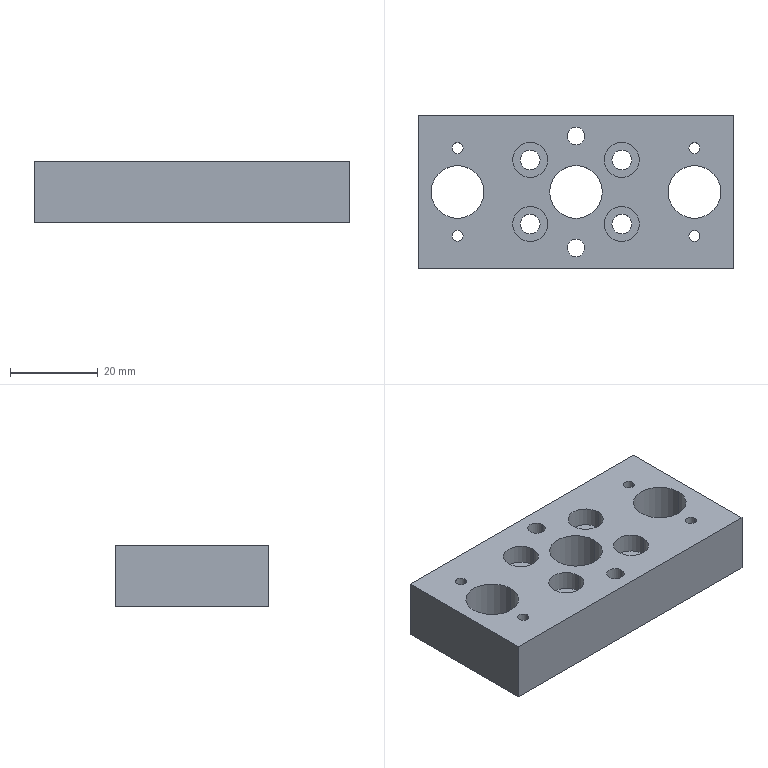Part | STEP file | 11-FG-SB01111 | 1 solid | 44 faces | box 72 x 35 x 14 mm | volume 28408 mm3 | cylinder 34 | plane 10 | commonest cylinder face diameters 2.5 x8 4.5 x8 8 x8 12 x6 4 x4
STEP:
#1=CARTESIAN_POINT('',(-6.,0.,0.));
#2=VERTEX_POINT('',#1);
#3=CARTESIAN_POINT('',(6.,0.,0.));
#4=VERTEX_POINT('',#3);
#5=CARTESIAN_POINT('',(0.,0.,0.));
#6=DIRECTION('',(0.,0.,1.));
#7=DIRECTION('',(1.,0.,0.));
#8=AXIS2_PLACEMENT_3D('',#5,#6,#7);
#9=CIRCLE('',#8,6.);
#10=EDGE_CURVE('',#2,#4,#9,.T.);
#11=ORIENTED_EDGE('',*,*,#10,.F.);
#12=CARTESIAN_POINT('',(-6.,0.,14.));
#13=VERTEX_POINT('',#12);
#14=CARTESIAN_POINT('',(-6.,0.,0.));
#15=DIRECTION('',(0.,0.,1.));
#16=VECTOR('',#15,1000.);
#17=LINE('',#14,#16);
#18=EDGE_CURVE('',#2,#13,#17,.T.);
#19=ORIENTED_EDGE('',*,*,#18,.T.);
#20=CARTESIAN_POINT('',(6.,0.,14.));
#21=VERTEX_POINT('',#20);
#22=CARTESIAN_POINT('',(0.,0.,14.));
#23=DIRECTION('',(0.,0.,1.));
#24=DIRECTION('',(1.,0.,0.));
#25=AXIS2_PLACEMENT_3D('',#22,#23,#24);
#26=CIRCLE('',#25,6.);
#27=EDGE_CURVE('',#13,#21,#26,.T.);
#28=ORIENTED_EDGE('',*,*,#27,.T.);
#29=CARTESIAN_POINT('',(6.,0.,0.));
#30=DIRECTION('',(0.,0.,1.));
#31=VECTOR('',#30,1000.);
#32=LINE('',#29,#31);
#33=EDGE_CURVE('',#4,#21,#32,.T.);
#34=ORIENTED_EDGE('',*,*,#33,.F.);
#35=EDGE_LOOP('',(#11,#19,#28,#34));
#36=FACE_OUTER_BOUND('',#35,.T.);
#37=CARTESIAN_POINT('',(0.,0.,0.));
#38=DIRECTION('',(0.,0.,1.));
#39=DIRECTION('',(1.,0.,0.));
#40=AXIS2_PLACEMENT_3D('',#37,#38,#39);
#41=CYLINDRICAL_SURFACE('',#40,6.);
#42=ADVANCED_FACE('',(#36),#41,.F.);
#43=CARTESIAN_POINT('',(28.25,10.,14.));
#44=VERTEX_POINT('',#43);
#45=CARTESIAN_POINT('',(25.75,10.,14.));
#46=VERTEX_POINT('',#45);
#47=CARTESIAN_POINT('',(27.,10.,14.));
#48=DIRECTION('',(0.,0.,-1.));
#49=DIRECTION('',(-1.,0.,0.));
#50=AXIS2_PLACEMENT_3D('',#47,#48,#49);
#51=CIRCLE('',#50,1.25);
#52=EDGE_CURVE('',#44,#46,#51,.T.);
#53=ORIENTED_EDGE('',*,*,#52,.F.);
#54=CARTESIAN_POINT('',(28.25,10.,0.));
#55=VERTEX_POINT('',#54);
#56=CARTESIAN_POINT('',(28.25,10.,0.));
#57=DIRECTION('',(0.,0.,-1.));
#58=VECTOR('',#57,1000.);
#59=LINE('',#56,#58);
#60=EDGE_CURVE('',#44,#55,#59,.T.);
#61=ORIENTED_EDGE('',*,*,#60,.T.);
#62=CARTESIAN_POINT('',(25.75,10.,0.));
#63=VERTEX_POINT('',#62);
#64=CARTESIAN_POINT('',(27.,10.,0.));
#65=DIRECTION('',(0.,0.,-1.));
#66=DIRECTION('',(-1.,0.,0.));
#67=AXIS2_PLACEMENT_3D('',#64,#65,#66);
#68=CIRCLE('',#67,1.25);
#69=EDGE_CURVE('',#55,#63,#68,.T.);
#70=ORIENTED_EDGE('',*,*,#69,.T.);
#71=CARTESIAN_POINT('',(25.75,10.,0.));
#72=DIRECTION('',(0.,0.,-1.));
#73=VECTOR('',#72,1000.);
#74=LINE('',#71,#73);
#75=EDGE_CURVE('',#46,#63,#74,.T.);
#76=ORIENTED_EDGE('',*,*,#75,.F.);
#77=EDGE_LOOP('',(#53,#61,#70,#76));
#78=FACE_OUTER_BOUND('',#77,.T.);
#79=CARTESIAN_POINT('',(27.,10.,0.));
#80=DIRECTION('',(0.,0.,-1.));
#81=DIRECTION('',(-1.,0.,0.));
#82=AXIS2_PLACEMENT_3D('',#79,#80,#81);
#83=CYLINDRICAL_SURFACE('',#82,1.25);
#84=ADVANCED_FACE('',(#78),#83,.F.);
#85=CARTESIAN_POINT('',(28.25,-10.018,14.));
#86=VERTEX_POINT('',#85);
#87=CARTESIAN_POINT('',(25.75,-10.018,14.));
#88=VERTEX_POINT('',#87);
#89=CARTESIAN_POINT('',(27.,-10.018,14.));
#90=DIRECTION('',(0.,0.,-1.));
#91=DIRECTION('',(-1.,0.,0.));
#92=AXIS2_PLACEMENT_3D('',#89,#90,#91);
#93=CIRCLE('',#92,1.25);
#94=EDGE_CURVE('',#86,#88,#93,.T.);
#95=ORIENTED_EDGE('',*,*,#94,.F.);
#96=CARTESIAN_POINT('',(28.25,-10.018,0.));
#97=VERTEX_POINT('',#96);
#98=CARTESIAN_POINT('',(28.25,-10.018,0.));
#99=DIRECTION('',(0.,0.,-1.));
#100=VECTOR('',#99,1000.);
#101=LINE('',#98,#100);
#102=EDGE_CURVE('',#86,#97,#101,.T.);
#103=ORIENTED_EDGE('',*,*,#102,.T.);
#104=CARTESIAN_POINT('',(25.75,-10.018,0.));
#105=VERTEX_POINT('',#104);
#106=CARTESIAN_POINT('',(27.,-10.018,0.));
#107=DIRECTION('',(0.,0.,-1.));
#108=DIRECTION('',(-1.,0.,0.));
#109=AXIS2_PLACEMENT_3D('',#106,#107,#108);
#110=CIRCLE('',#109,1.25);
#111=EDGE_CURVE('',#97,#105,#110,.T.);
#112=ORIENTED_EDGE('',*,*,#111,.T.);
#113=CARTESIAN_POINT('',(25.75,-10.018,0.));
#114=DIRECTION('',(0.,0.,-1.));
#115=VECTOR('',#114,1000.);
#116=LINE('',#113,#115);
#117=EDGE_CURVE('',#88,#105,#116,.T.);
#118=ORIENTED_EDGE('',*,*,#117,.F.);
#119=EDGE_LOOP('',(#95,#103,#112,#118));
#120=FACE_OUTER_BOUND('',#119,.T.);
#121=CARTESIAN_POINT('',(27.,-10.018,0.));
#122=DIRECTION('',(0.,0.,-1.));
#123=DIRECTION('',(-1.,0.,0.));
#124=AXIS2_PLACEMENT_3D('',#121,#122,#123);
#125=CYLINDRICAL_SURFACE('',#124,1.25);
#126=ADVANCED_FACE('',(#120),#125,.F.);
#127=CARTESIAN_POINT('',(-25.75,10.,14.));
#128=VERTEX_POINT('',#127);
#129=CARTESIAN_POINT('',(-28.25,10.,14.));
#130=VERTEX_POINT('',#129);
#131=CARTESIAN_POINT('',(-27.,10.,14.));
#132=DIRECTION('',(0.,0.,-1.));
#133=DIRECTION('',(-1.,0.,0.));
#134=AXIS2_PLACEMENT_3D('',#131,#132,#133);
#135=CIRCLE('',#134,1.25);
#136=EDGE_CURVE('',#128,#130,#135,.T.);
#137=ORIENTED_EDGE('',*,*,#136,.F.);
#138=CARTESIAN_POINT('',(-25.75,10.,0.));
#139=VERTEX_POINT('',#138);
#140=CARTESIAN_POINT('',(-25.75,10.,0.));
#141=DIRECTION('',(0.,0.,-1.));
#142=VECTOR('',#141,1000.);
#143=LINE('',#140,#142);
#144=EDGE_CURVE('',#128,#139,#143,.T.);
#145=ORIENTED_EDGE('',*,*,#144,.T.);
#146=CARTESIAN_POINT('',(-28.25,10.,0.));
#147=VERTEX_POINT('',#146);
#148=CARTESIAN_POINT('',(-27.,10.,0.));
#149=DIRECTION('',(0.,0.,-1.));
#150=DIRECTION('',(-1.,0.,0.));
#151=AXIS2_PLACEMENT_3D('',#148,#149,#150);
#152=CIRCLE('',#151,1.25);
#153=EDGE_CURVE('',#139,#147,#152,.T.);
#154=ORIENTED_EDGE('',*,*,#153,.T.);
#155=CARTESIAN_POINT('',(-28.25,10.,0.));
#156=DIRECTION('',(0.,0.,-1.));
#157=VECTOR('',#156,1000.);
#158=LINE('',#155,#157);
#159=EDGE_CURVE('',#130,#147,#158,.T.);
#160=ORIENTED_EDGE('',*,*,#159,.F.);
#161=EDGE_LOOP('',(#137,#145,#154,#160));
#162=FACE_OUTER_BOUND('',#161,.T.);
#163=CARTESIAN_POINT('',(-27.,10.,0.));
#164=DIRECTION('',(0.,0.,-1.));
#165=DIRECTION('',(-1.,0.,0.));
#166=AXIS2_PLACEMENT_3D('',#163,#164,#165);
#167=CYLINDRICAL_SURFACE('',#166,1.25);
#168=ADVANCED_FACE('',(#162),#167,.F.);
#169=CARTESIAN_POINT('',(-25.75,-10.,14.));
#170=VERTEX_POINT('',#169);
#171=CARTESIAN_POINT('',(-28.25,-10.,14.));
#172=VERTEX_POINT('',#171);
#173=CARTESIAN_POINT('',(-27.,-10.,14.));
#174=DIRECTION('',(0.,0.,-1.));
#175=DIRECTION('',(-1.,0.,0.));
#176=AXIS2_PLACEMENT_3D('',#173,#174,#175);
#177=CIRCLE('',#176,1.25);
#178=EDGE_CURVE('',#170,#172,#177,.T.);
#179=ORIENTED_EDGE('',*,*,#178,.F.);
#180=CARTESIAN_POINT('',(-25.75,-10.,0.));
#181=VERTEX_POINT('',#180);
#182=CARTESIAN_POINT('',(-25.75,-10.,0.));
#183=DIRECTION('',(0.,0.,-1.));
#184=VECTOR('',#183,1000.);
#185=LINE('',#182,#184);
#186=EDGE_CURVE('',#170,#181,#185,.T.);
#187=ORIENTED_EDGE('',*,*,#186,.T.);
#188=CARTESIAN_POINT('',(-28.25,-10.,0.));
#189=VERTEX_POINT('',#188);
#190=CARTESIAN_POINT('',(-27.,-10.,0.));
#191=DIRECTION('',(0.,0.,-1.));
#192=DIRECTION('',(-1.,0.,0.));
#193=AXIS2_PLACEMENT_3D('',#190,#191,#192);
#194=CIRCLE('',#193,1.25);
#195=EDGE_CURVE('',#181,#189,#194,.T.);
#196=ORIENTED_EDGE('',*,*,#195,.T.);
#197=CARTESIAN_POINT('',(-28.25,-10.,0.));
#198=DIRECTION('',(0.,0.,-1.));
#199=VECTOR('',#198,1000.);
#200=LINE('',#197,#199);
#201=EDGE_CURVE('',#172,#189,#200,.T.);
#202=ORIENTED_EDGE('',*,*,#201,.F.);
#203=EDGE_LOOP('',(#179,#187,#196,#202));
#204=FACE_OUTER_BOUND('',#203,.T.);
#205=CARTESIAN_POINT('',(-27.,-10.,0.));
#206=DIRECTION('',(0.,0.,-1.));
#207=DIRECTION('',(-1.,0.,0.));
#208=AXIS2_PLACEMENT_3D('',#205,#206,#207);
#209=CYLINDRICAL_SURFACE('',#208,1.25);
#210=ADVANCED_FACE('',(#204),#209,.F.);
#211=CARTESIAN_POINT('',(-21.,0.,14.));
#212=VERTEX_POINT('',#211);
#213=CARTESIAN_POINT('',(-33.,0.,14.));
#214=VERTEX_POINT('',#213);
#215=CARTESIAN_POINT('',(-27.,0.,14.));
#216=DIRECTION('',(0.,0.,-1.));
#217=DIRECTION('',(1.,0.,0.));
#218=AXIS2_PLACEMENT_3D('',#215,#216,#217);
#219=CIRCLE('',#218,6.);
#220=EDGE_CURVE('',#212,#214,#219,.T.);
#221=ORIENTED_EDGE('',*,*,#220,.F.);
#222=CARTESIAN_POINT('',(-21.,0.,0.));
#223=VERTEX_POINT('',#222);
#224=CARTESIAN_POINT('',(-21.,0.,14.));
#225=DIRECTION('',(0.,0.,-1.));
#226=VECTOR('',#225,1000.);
#227=LINE('',#224,#226);
#228=EDGE_CURVE('',#212,#223,#227,.T.);
#229=ORIENTED_EDGE('',*,*,#228,.T.);
#230=CARTESIAN_POINT('',(-33.,0.,0.));
#231=VERTEX_POINT('',#230);
#232=CARTESIAN_POINT('',(-27.,0.,0.));
#233=DIRECTION('',(0.,0.,-1.));
#234=DIRECTION('',(1.,0.,0.));
#235=AXIS2_PLACEMENT_3D('',#232,#233,#234);
#236=CIRCLE('',#235,6.);
#237=EDGE_CURVE('',#223,#231,#236,.T.);
#238=ORIENTED_EDGE('',*,*,#237,.T.);
#239=CARTESIAN_POINT('',(-33.,0.,14.));
#240=DIRECTION('',(0.,0.,-1.));
#241=VECTOR('',#240,1000.);
#242=LINE('',#239,#241);
#243=EDGE_CURVE('',#214,#231,#242,.T.);
#244=ORIENTED_EDGE('',*,*,#243,.F.);
#245=EDGE_LOOP('',(#221,#229,#238,#244));
#246=FACE_OUTER_BOUND('',#245,.T.);
#247=CARTESIAN_POINT('',(-27.,0.,14.));
#248=DIRECTION('',(0.,0.,-1.));
#249=DIRECTION('',(-1.,0.,0.));
#250=AXIS2_PLACEMENT_3D('',#247,#248,#249);
#251=CYLINDRICAL_SURFACE('',#250,6.);
#252=ADVANCED_FACE('',(#246),#251,.F.);
#253=CARTESIAN_POINT('',(33.,0.,14.));
#254=VERTEX_POINT('',#253);
#255=CARTESIAN_POINT('',(21.,0.,14.));
#256=VERTEX_POINT('',#255);
#257=CARTESIAN_POINT('',(27.,0.,14.));
#258=DIRECTION('',(0.,0.,-1.));
#259=DIRECTION('',(-1.,0.,0.));
#260=AXIS2_PLACEMENT_3D('',#257,#258,#259);
#261=CIRCLE('',#260,6.);
#262=EDGE_CURVE('',#254,#256,#261,.T.);
#263=ORIENTED_EDGE('',*,*,#262,.F.);
#264=CARTESIAN_POINT('',(33.,0.,0.));
#265=VERTEX_POINT('',#264);
#266=CARTESIAN_POINT('',(33.,0.,14.));
#267=DIRECTION('',(0.,0.,-1.));
#268=VECTOR('',#267,1000.);
#269=LINE('',#266,#268);
#270=EDGE_CURVE('',#254,#265,#269,.T.);
#271=ORIENTED_EDGE('',*,*,#270,.T.);
#272=CARTESIAN_POINT('',(21.,0.,0.));
#273=VERTEX_POINT('',#272);
#274=CARTESIAN_POINT('',(27.,0.,0.));
#275=DIRECTION('',(0.,0.,-1.));
#276=DIRECTION('',(-1.,0.,0.));
#277=AXIS2_PLACEMENT_3D('',#274,#275,#276);
#278=CIRCLE('',#277,6.);
#279=EDGE_CURVE('',#265,#273,#278,.T.);
#280=ORIENTED_EDGE('',*,*,#279,.T.);
#281=CARTESIAN_POINT('',(21.,0.,14.));
#282=DIRECTION('',(0.,0.,-1.));
#283=VECTOR('',#282,1000.);
#284=LINE('',#281,#283);
#285=EDGE_CURVE('',#256,#273,#284,.T.);
#286=ORIENTED_EDGE('',*,*,#285,.F.);
#287=EDGE_LOOP('',(#263,#271,#280,#286));
#288=FACE_OUTER_BOUND('',#287,.T.);
#289=CARTESIAN_POINT('',(27.,0.,14.));
#290=DIRECTION('',(0.,0.,-1.));
#291=DIRECTION('',(-1.,0.,0.));
#292=AXIS2_PLACEMENT_3D('',#289,#290,#291);
#293=CYLINDRICAL_SURFACE('',#292,6.);
#294=ADVANCED_FACE('',(#288),#293,.F.);
#295=CARTESIAN_POINT('',(6.444,-7.313,9.6));
#296=VERTEX_POINT('',#295);
#297=CARTESIAN_POINT('',(14.444,-7.313,9.6));
#298=VERTEX_POINT('',#297);
#299=CARTESIAN_POINT('',(10.444,-7.313,9.6));
#300=DIRECTION('',(0.,0.,1.));
#301=DIRECTION('',(1.,0.,0.));
#302=AXIS2_PLACEMENT_3D('',#299,#300,#301);
#303=CIRCLE('',#302,4.);
#304=EDGE_CURVE('',#296,#298,#303,.T.);
#305=ORIENTED_EDGE('',*,*,#304,.F.);
#306=CARTESIAN_POINT('',(6.444,-7.313,14.));
#307=VERTEX_POINT('',#306);
#308=CARTESIAN_POINT('',(6.444,-7.313,14.));
#309=DIRECTION('',(0.,0.,1.));
#310=VECTOR('',#309,1000.);
#311=LINE('',#308,#310);
#312=EDGE_CURVE('',#296,#307,#311,.T.);
#313=ORIENTED_EDGE('',*,*,#312,.T.);
#314=CARTESIAN_POINT('',(14.444,-7.313,14.));
#315=VERTEX_POINT('',#314);
#316=CARTESIAN_POINT('',(10.444,-7.313,14.));
#317=DIRECTION('',(0.,0.,1.));
#318=DIRECTION('',(1.,0.,0.));
#319=AXIS2_PLACEMENT_3D('',#316,#317,#318);
#320=CIRCLE('',#319,4.);
#321=EDGE_CURVE('',#307,#315,#320,.T.);
#322=ORIENTED_EDGE('',*,*,#321,.T.);
#323=CARTESIAN_POINT('',(14.444,-7.313,14.));
#324=DIRECTION('',(0.,0.,1.));
#325=VECTOR('',#324,1000.);
#326=LINE('',#323,#325);
#327=EDGE_CURVE('',#298,#315,#326,.T.);
#328=ORIENTED_EDGE('',*,*,#327,.F.);
#329=EDGE_LOOP('',(#305,#313,#322,#328));
#330=FACE_OUTER_BOUND('',#329,.T.);
#331=CARTESIAN_POINT('',(10.444,-7.313,14.));
#332=DIRECTION('',(0.,0.,1.));
#333=DIRECTION('',(1.,0.,0.));
#334=AXIS2_PLACEMENT_3D('',#331,#332,#333);
#335=CYLINDRICAL_SURFACE('',#334,4.);
#336=ADVANCED_FACE('',(#330),#335,.F.);
#337=CARTESIAN_POINT('',(8.194,-7.313,0.));
#338=VERTEX_POINT('',#337);
#339=CARTESIAN_POINT('',(12.694,-7.313,0.));
#340=VERTEX_POINT('',#339);
#341=CARTESIAN_POINT('',(10.444,-7.313,0.));
#342=DIRECTION('',(0.,0.,1.));
#343=DIRECTION('',(1.,0.,0.));
#344=AXIS2_PLACEMENT_3D('',#341,#342,#343);
#345=CIRCLE('',#344,2.25);
#346=EDGE_CURVE('',#338,#340,#345,.T.);
#347=ORIENTED_EDGE('',*,*,#346,.F.);
#348=CARTESIAN_POINT('',(8.194,-7.313,9.6));
#349=VERTEX_POINT('',#348);
#350=CARTESIAN_POINT('',(8.194,-7.313,14.));
#351=DIRECTION('',(0.,0.,1.));
#352=VECTOR('',#351,1000.);
#353=LINE('',#350,#352);
#354=EDGE_CURVE('',#338,#349,#353,.T.);
#355=ORIENTED_EDGE('',*,*,#354,.T.);
#356=CARTESIAN_POINT('',(12.694,-7.313,9.6));
#357=VERTEX_POINT('',#356);
#358=CARTESIAN_POINT('',(10.444,-7.313,9.6));
#359=DIRECTION('',(0.,0.,1.));
#360=DIRECTION('',(1.,0.,0.));
#361=AXIS2_PLACEMENT_3D('',#358,#359,#360);
#362=CIRCLE('',#361,2.25);
#363=EDGE_CURVE('',#349,#357,#362,.T.);
#364=ORIENTED_EDGE('',*,*,#363,.T.);
#365=CARTESIAN_POINT('',(12.694,-7.313,14.));
#366=DIRECTION('',(0.,0.,1.));
#367=VECTOR('',#366,1000.);
#368=LINE('',#365,#367);
#369=EDGE_CURVE('',#340,#357,#368,.T.);
#370=ORIENTED_EDGE('',*,*,#369,.F.);
#371=EDGE_LOOP('',(#347,#355,#364,#370));
#372=FACE_OUTER_BOUND('',#371,.T.);
#373=CARTESIAN_POINT('',(10.444,-7.313,14.));
#374=DIRECTION('',(0.,0.,1.));
#375=DIRECTION('',(1.,0.,0.));
#376=AXIS2_PLACEMENT_3D('',#373,#374,#375);
#377=CYLINDRICAL_SURFACE('',#376,2.25);
#378=ADVANCED_FACE('',(#372),#377,.F.);
#379=CARTESIAN_POINT('',(-14.444,7.313,9.6));
#380=VERTEX_POINT('',#379);
#381=CARTESIAN_POINT('',(-6.444,7.313,9.6));
#382=VERTEX_POINT('',#381);
#383=CARTESIAN_POINT('',(-10.444,7.313,9.6));
#384=DIRECTION('',(0.,0.,1.));
#385=DIRECTION('',(1.,0.,0.));
#386=AXIS2_PLACEMENT_3D('',#383,#384,#385);
#387=CIRCLE('',#386,4.);
#388=EDGE_CURVE('',#380,#382,#387,.T.);
#389=ORIENTED_EDGE('',*,*,#388,.F.);
#390=CARTESIAN_POINT('',(-14.444,7.313,14.));
#391=VERTEX_POINT('',#390);
#392=CARTESIAN_POINT('',(-14.444,7.313,14.));
#393=DIRECTION('',(0.,0.,1.));
#394=VECTOR('',#393,1000.);
#395=LINE('',#392,#394);
#396=EDGE_CURVE('',#380,#391,#395,.T.);
#397=ORIENTED_EDGE('',*,*,#396,.T.);
#398=CARTESIAN_POINT('',(-6.444,7.313,14.));
#399=VERTEX_POINT('',#398);
#400=CARTESIAN_POINT('',(-10.444,7.313,14.));
#401=DIRECTION('',(0.,0.,1.));
#402=DIRECTION('',(1.,0.,0.));
#403=AXIS2_PLACEMENT_3D('',#400,#401,#402);
#404=CIRCLE('',#403,4.);
#405=EDGE_CURVE('',#391,#399,#404,.T.);
#406=ORIENTED_EDGE('',*,*,#405,.T.);
#407=CARTESIAN_POINT('',(-6.444,7.313,14.));
#408=DIRECTION('',(0.,0.,1.));
#409=VECTOR('',#408,1000.);
#410=LINE('',#407,#409);
#411=EDGE_CURVE('',#382,#399,#410,.T.);
#412=ORIENTED_EDGE('',*,*,#411,.F.);
#413=EDGE_LOOP('',(#389,#397,#406,#412));
#414=FACE_OUTER_BOUND('',#413,.T.);
#415=CARTESIAN_POINT('',(-10.444,7.313,14.));
#416=DIRECTION('',(0.,0.,1.));
#417=DIRECTION('',(1.,0.,0.));
#418=AXIS2_PLACEMENT_3D('',#415,#416,#417);
#419=CYLINDRICAL_SURFACE('',#418,4.);
#420=ADVANCED_FACE('',(#414),#419,.F.);
#421=CARTESIAN_POINT('',(-12.694,7.313,0.));
#422=VERTEX_POINT('',#421);
#423=CARTESIAN_POINT('',(-8.194,7.313,0.));
#424=VERTEX_POINT('',#423);
#425=CARTESIAN_POINT('',(-10.444,7.313,0.));
#426=DIRECTION('',(0.,0.,1.));
#427=DIRECTION('',(1.,0.,0.));
#428=AXIS2_PLACEMENT_3D('',#425,#426,#427);
#429=CIRCLE('',#428,2.25);
#430=EDGE_CURVE('',#422,#424,#429,.T.);
#431=ORIENTED_EDGE('',*,*,#430,.F.);
#432=CARTESIAN_POINT('',(-12.694,7.313,9.6));
#433=VERTEX_POINT('',#432);
#434=CARTESIAN_POINT('',(-12.694,7.313,14.));
#435=DIRECTION('',(0.,0.,1.));
#436=VECTOR('',#435,1000.);
#437=LINE('',#434,#436);
#438=EDGE_CURVE('',#422,#433,#437,.T.);
#439=ORIENTED_EDGE('',*,*,#438,.T.);
#440=CARTESIAN_POINT('',(-8.194,7.313,9.6));
#441=VERTEX_POINT('',#440);
#442=CARTESIAN_POINT('',(-10.444,7.313,9.6));
#443=DIRECTION('',(0.,0.,1.));
#444=DIRECTION('',(1.,0.,0.));
#445=AXIS2_PLACEMENT_3D('',#442,#443,#444);
#446=CIRCLE('',#445,2.25);
#447=EDGE_CURVE('',#433,#441,#446,.T.);
#448=ORIENTED_EDGE('',*,*,#447,.T.);
#449=CARTESIAN_POINT('',(-8.194,7.313,14.));
#450=DIRECTION('',(0.,0.,1.));
#451=VECTOR('',#450,1000.);
#452=LINE('',#449,#451);
#453=EDGE_CURVE('',#424,#441,#452,.T.);
#454=ORIENTED_EDGE('',*,*,#453,.F.);
#455=EDGE_LOOP('',(#431,#439,#448,#454));
#456=FACE_OUTER_BOUND('',#455,.T.);
#457=CARTESIAN_POINT('',(-10.444,7.313,14.));
#458=DIRECTION('',(0.,0.,1.));
#459=DIRECTION('',(1.,0.,0.));
#460=AXIS2_PLACEMENT_3D('',#457,#458,#459);
#461=CYLINDRICAL_SURFACE('',#460,2.25);
#462=ADVANCED_FACE('',(#456),#461,.F.);
#463=CARTESIAN_POINT('',(-14.444,-7.313,9.6));
#464=VERTEX_POINT('',#463);
#465=CARTESIAN_POINT('',(-6.444,-7.313,9.6));
#466=VERTEX_POINT('',#465);
#467=CARTESIAN_POINT('',(-10.444,-7.313,9.6));
#468=DIRECTION('',(0.,0.,1.));
#469=DIRECTION('',(1.,0.,0.));
#470=AXIS2_PLACEMENT_3D('',#467,#468,#469);
#471=CIRCLE('',#470,4.);
#472=EDGE_CURVE('',#464,#466,#471,.T.);
#473=ORIENTED_EDGE('',*,*,#472,.F.);
#474=CARTESIAN_POINT('',(-14.444,-7.313,14.));
#475=VERTEX_POINT('',#474);
#476=CARTESIAN_POINT('',(-14.444,-7.313,14.));
#477=DIRECTION('',(0.,0.,1.));
#478=VECTOR('',#477,1000.);
#479=LINE('',#476,#478);
#480=EDGE_CURVE('',#464,#475,#479,.T.);
#481=ORIENTED_EDGE('',*,*,#480,.T.);
#482=CARTESIAN_POINT('',(-6.444,-7.313,14.));
#483=VERTEX_POINT('',#482);
#484=CARTESIAN_POINT('',(-10.444,-7.313,14.));
#485=DIRECTION('',(0.,0.,1.));
#486=DIRECTION('',(1.,0.,0.));
#487=AXIS2_PLACEMENT_3D('',#484,#485,#486);
#488=CIRCLE('',#487,4.);
#489=EDGE_CURVE('',#475,#483,#488,.T.);
#490=ORIENTED_EDGE('',*,*,#489,.T.);
#491=CARTESIAN_POINT('',(-6.444,-7.313,14.));
#492=DIRECTION('',(0.,0.,1.));
#493=VECTOR('',#492,1000.);
#494=LINE('',#491,#493);
#495=EDGE_CURVE('',#466,#483,#494,.T.);
#496=ORIENTED_EDGE('',*,*,#495,.F.);
#497=EDGE_LOOP('',(#473,#481,#490,#496));
#498=FACE_OUTER_BOUND('',#497,.T.);
#499=CARTESIAN_POINT('',(-10.444,-7.313,14.));
#500=DIRECTION('',(0.,0.,1.));
#501=DIRECTION('',(1.,0.,0.));
#502=AXIS2_PLACEMENT_3D('',#499,#500,#501);
#503=CYLINDRICAL_SURFACE('',#502,4.);
#504=ADVANCED_FACE('',(#498),#503,.F.);
#505=CARTESIAN_POINT('',(-12.694,-7.313,0.));
#506=VERTEX_POINT('',#505);
#507=CARTESIAN_POINT('',(-8.194,-7.313,0.));
#508=VERTEX_POINT('',#507);
#509=CARTESIAN_POINT('',(-10.444,-7.313,0.));
#510=DIRECTION('',(0.,0.,1.));
#511=DIRECTION('',(1.,0.,0.));
#512=AXIS2_PLACEMENT_3D('',#509,#510,#511);
#513=CIRCLE('',#512,2.25);
#514=EDGE_CURVE('',#506,#508,#513,.T.);
#515=ORIENTED_EDGE('',*,*,#514,.F.);
#516=CARTESIAN_POINT('',(-12.694,-7.313,9.6));
#517=VERTEX_POINT('',#516);
#518=CARTESIAN_POINT('',(-12.694,-7.313,14.));
#519=DIRECTION('',(0.,0.,1.));
#520=VECTOR('',#519,1000.);
#521=LINE('',#518,#520);
#522=EDGE_CURVE('',#506,#517,#521,.T.);
#523=ORIENTED_EDGE('',*,*,#522,.T.);
#524=CARTESIAN_POINT('',(-8.194,-7.313,9.6));
#525=VERTEX_POINT('',#524);
#526=CARTESIAN_POINT('',(-10.444,-7.313,9.6));
#527=DIRECTION('',(0.,0.,1.));
#528=DIRECTION('',(1.,0.,0.));
#529=AXIS2_PLACEMENT_3D('',#526,#527,#528);
#530=CIRCLE('',#529,2.25);
#531=EDGE_CURVE('',#517,#525,#530,.T.);
#532=ORIENTED_EDGE('',*,*,#531,.T.);
#533=CARTESIAN_POINT('',(-8.194,-7.313,14.));
#534=DIRECTION('',(0.,0.,1.));
#535=VECTOR('',#534,1000.);
#536=LINE('',#533,#535);
#537=EDGE_CURVE('',#508,#525,#536,.T.);
#538=ORIENTED_EDGE('',*,*,#537,.F.);
#539=EDGE_LOOP('',(#515,#523,#532,#538));
#540=FACE_OUTER_BOUND('',#539,.T.);
#541=CARTESIAN_POINT('',(-10.444,-7.313,14.));
#542=DIRECTION('',(0.,0.,1.));
#543=DIRECTION('',(1.,0.,0.));
#544=AXIS2_PLACEMENT_3D('',#541,#542,#543);
#545=CYLINDRICAL_SURFACE('',#544,2.25);
#546=ADVANCED_FACE('',(#540),#545,.F.);
#547=CARTESIAN_POINT('',(6.444,7.313,9.6));
#548=VERTEX_POINT('',#547);
#549=CARTESIAN_POINT('',(14.444,7.313,9.6));
#550=VERTEX_POINT('',#549);
#551=CARTESIAN_POINT('',(10.444,7.313,9.6));
#552=DIRECTION('',(0.,0.,1.));
#553=DIRECTION('',(1.,0.,0.));
#554=AXIS2_PLACEMENT_3D('',#551,#552,#553);
#555=CIRCLE('',#554,4.);
#556=EDGE_CURVE('',#548,#550,#555,.T.);
#557=ORIENTED_EDGE('',*,*,#556,.F.);
#558=CARTESIAN_POINT('',(6.444,7.313,14.));
#559=VERTEX_POINT('',#558);
#560=CARTESIAN_POINT('',(6.444,7.313,14.));
#561=DIRECTION('',(0.,0.,1.));
#562=VECTOR('',#561,1000.);
#563=LINE('',#560,#562);
#564=EDGE_CURVE('',#548,#559,#563,.T.);
#565=ORIENTED_EDGE('',*,*,#564,.T.);
#566=CARTESIAN_POINT('',(14.444,7.313,14.));
#567=VERTEX_POINT('',#566);
#568=CARTESIAN_POINT('',(10.444,7.313,14.));
#569=DIRECTION('',(0.,0.,1.));
#570=DIRECTION('',(1.,0.,0.));
#571=AXIS2_PLACEMENT_3D('',#568,#569,#570);
#572=CIRCLE('',#571,4.);
#573=EDGE_CURVE('',#559,#567,#572,.T.);
#574=ORIENTED_EDGE('',*,*,#573,.T.);
#575=CARTESIAN_POINT('',(14.444,7.313,14.));
#576=DIRECTION('',(0.,0.,1.));
#577=VECTOR('',#576,1000.);
#578=LINE('',#575,#577);
#579=EDGE_CURVE('',#550,#567,#578,.T.);
#580=ORIENTED_EDGE('',*,*,#579,.F.);
#581=EDGE_LOOP('',(#557,#565,#574,#580));
#582=FACE_OUTER_BOUND('',#581,.T.);
#583=CARTESIAN_POINT('',(10.444,7.313,14.));
#584=DIRECTION('',(0.,0.,1.));
#585=DIRECTION('',(1.,0.,0.));
#586=AXIS2_PLACEMENT_3D('',#583,#584,#585);
#587=CYLINDRICAL_SURFACE('',#586,4.);
#588=ADVANCED_FACE('',(#582),#587,.F.);
#589=CARTESIAN_POINT('',(8.194,7.313,0.));
#590=VERTEX_POINT('',#589);
#591=CARTESIAN_POINT('',(12.694,7.313,0.));
#592=VERTEX_POINT('',#591);
#593=CARTESIAN_POINT('',(10.444,7.313,0.));
#594=DIRECTION('',(0.,0.,1.));
#595=DIRECTION('',(1.,0.,0.));
#596=AXIS2_PLACEMENT_3D('',#593,#594,#595);
#597=CIRCLE('',#596,2.25);
#598=EDGE_CURVE('',#590,#592,#597,.T.);
#599=ORIENTED_EDGE('',*,*,#598,.F.);
#600=CARTESIAN_POINT('',(8.194,7.313,9.6));
#601=VERTEX_POINT('',#600);
#602=CARTESIAN_POINT('',(8.194,7.313,14.));
#603=DIRECTION('',(0.,0.,1.));
#604=VECTOR('',#603,1000.);
#605=LINE('',#602,#604);
#606=EDGE_CURVE('',#590,#601,#605,.T.);
#607=ORIENTED_EDGE('',*,*,#606,.T.);
#608=CARTESIAN_POINT('',(12.694,7.313,9.6));
#609=VERTEX_POINT('',#608);
#610=CARTESIAN_POINT('',(10.444,7.313,9.6));
#611=DIRECTION('',(0.,0.,1.));
#612=DIRECTION('',(1.,0.,0.));
#613=AXIS2_PLACEMENT_3D('',#610,#611,#612);
#614=CIRCLE('',#613,2.25);
#615=EDGE_CURVE('',#601,#609,#614,.T.);
#616=ORIENTED_EDGE('',*,*,#615,.T.);
#617=CARTESIAN_POINT('',(12.694,7.313,14.));
#618=DIRECTION('',(0.,0.,1.));
#619=VECTOR('',#618,1000.);
#620=LINE('',#617,#619);
#621=EDGE_CURVE('',#592,#609,#620,.T.);
#622=ORIENTED_EDGE('',*,*,#621,.F.);
#623=EDGE_LOOP('',(#599,#607,#616,#622));
#624=FACE_OUTER_BOUND('',#623,.T.);
#625=CARTESIAN_POINT('',(10.444,7.313,14.));
#626=DIRECTION('',(0.,0.,1.));
#627=DIRECTION('',(1.,0.,0.));
#628=AXIS2_PLACEMENT_3D('',#625,#626,#627);
#629=CYLINDRICAL_SURFACE('',#628,2.25);
#630=ADVANCED_FACE('',(#624),#629,.F.);
#631=CARTESIAN_POINT('',(-2.,-12.75,0.));
#632=VERTEX_POINT('',#631);
#633=CARTESIAN_POINT('',(2.,-12.75,0.));
#634=VERTEX_POINT('',#633);
#635=CARTESIAN_POINT('',(0.,-12.75,0.));
#636=DIRECTION('',(0.,0.,1.));
#637=DIRECTION('',(1.,0.,0.));
#638=AXIS2_PLACEMENT_3D('',#635,#636,#637);
#639=CIRCLE('',#638,2.);
#640=EDGE_CURVE('',#632,#634,#639,.T.);
#641=ORIENTED_EDGE('',*,*,#640,.F.);
#642=CARTESIAN_POINT('',(-2.,-12.75,14.));
#643=VERTEX_POINT('',#642);
#644=CARTESIAN_POINT('',(-2.,-12.75,14.));
#645=DIRECTION('',(0.,0.,1.));
#646=VECTOR('',#645,1000.);
#647=LINE('',#644,#646);
#648=EDGE_CURVE('',#632,#643,#647,.T.);
#649=ORIENTED_EDGE('',*,*,#648,.T.);
#650=CARTESIAN_POINT('',(2.,-12.75,14.));
#651=VERTEX_POINT('',#650);
#652=CARTESIAN_POINT('',(0.,-12.75,14.));
#653=DIRECTION('',(0.,0.,1.));
#654=DIRECTION('',(1.,0.,0.));
#655=AXIS2_PLACEMENT_3D('',#652,#653,#654);
#656=CIRCLE('',#655,2.);
#657=EDGE_CURVE('',#643,#651,#656,.T.);
#658=ORIENTED_EDGE('',*,*,#657,.T.);
#659=CARTESIAN_POINT('',(2.,-12.75,14.));
#660=DIRECTION('',(0.,0.,1.));
#661=VECTOR('',#660,1000.);
#662=LINE('',#659,#661);
#663=EDGE_CURVE('',#634,#651,#662,.T.);
#664=ORIENTED_EDGE('',*,*,#663,.F.);
#665=EDGE_LOOP('',(#641,#649,#658,#664));
#666=FACE_OUTER_BOUND('',#665,.T.);
#667=CARTESIAN_POINT('',(0.,-12.75,14.));
#668=DIRECTION('',(0.,0.,1.));
#669=DIRECTION('',(1.,0.,0.));
#670=AXIS2_PLACEMENT_3D('',#667,#668,#669);
#671=CYLINDRICAL_SURFACE('',#670,2.);
#672=ADVANCED_FACE('',(#666),#671,.F.);
#673=CARTESIAN_POINT('',(-2.,12.75,0.));
#674=VERTEX_POINT('',#673);
#675=CARTESIAN_POINT('',(2.,12.75,0.));
#676=VERTEX_POINT('',#675);
#677=CARTESIAN_POINT('',(0.,12.75,0.));
#678=DIRECTION('',(0.,0.,1.));
#679=DIRECTION('',(1.,0.,0.));
#680=AXIS2_PLACEMENT_3D('',#677,#678,#679);
#681=CIRCLE('',#680,2.);
#682=EDGE_CURVE('',#674,#676,#681,.T.);
#683=ORIENTED_EDGE('',*,*,#682,.F.);
#684=CARTESIAN_POINT('',(-2.,12.75,14.));
#685=VERTEX_POINT('',#684);
#686=CARTESIAN_POINT('',(-2.,12.75,14.));
#687=DIRECTION('',(0.,0.,1.));
#688=VECTOR('',#687,1000.);
#689=LINE('',#686,#688);
#690=EDGE_CURVE('',#674,#685,#689,.T.);
#691=ORIENTED_EDGE('',*,*,#690,.T.);
#692=CARTESIAN_POINT('',(2.,12.75,14.));
#693=VERTEX_POINT('',#692);
#694=CARTESIAN_POINT('',(0.,12.75,14.));
#695=DIRECTION('',(0.,0.,1.));
#696=DIRECTION('',(1.,0.,0.));
#697=AXIS2_PLACEMENT_3D('',#694,#695,#696);
#698=CIRCLE('',#697,2.);
#699=EDGE_CURVE('',#685,#693,#698,.T.);
#700=ORIENTED_EDGE('',*,*,#699,.T.);
#701=CARTESIAN_POINT('',(2.,12.75,14.));
#702=DIRECTION('',(0.,0.,1.));
#703=VECTOR('',#702,1000.);
#704=LINE('',#701,#703);
#705=EDGE_CURVE('',#676,#693,#704,.T.);
#706=ORIENTED_EDGE('',*,*,#705,.F.);
#707=EDGE_LOOP('',(#683,#691,#700,#706));
#708=FACE_OUTER_BOUND('',#707,.T.);
#709=CARTESIAN_POINT('',(0.,12.75,14.));
#710=DIRECTION('',(0.,0.,1.));
#711=DIRECTION('',(1.,0.,0.));
#712=AXIS2_PLACEMENT_3D('',#709,#710,#711);
#713=CYLINDRICAL_SURFACE('',#712,2.);
#714=ADVANCED_FACE('',(#708),#713,.F.);
#715=CARTESIAN_POINT('',(36.,-17.5,0.));
#716=VERTEX_POINT('',#715);
#717=CARTESIAN_POINT('',(36.,17.5,0.));
#718=VERTEX_POINT('',#717);
#719=CARTESIAN_POINT('',(36.,17.5,0.));
#720=DIRECTION('',(0.,1.,0.));
#721=VECTOR('',#720,1000.);
#722=LINE('',#719,#721);
#723=EDGE_CURVE('',#716,#718,#722,.T.);
#724=ORIENTED_EDGE('',*,*,#723,.T.);
#725=CARTESIAN_POINT('',(36.,17.5,14.));
#726=VERTEX_POINT('',#725);
#727=CARTESIAN_POINT('',(36.,17.5,14.));
#728=DIRECTION('',(0.,0.,-1.));
#729=VECTOR('',#728,1000.);
#730=LINE('',#727,#729);
#731=EDGE_CURVE('',#726,#718,#730,.T.);
#732=ORIENTED_EDGE('',*,*,#731,.F.);
#733=CARTESIAN_POINT('',(36.,-17.5,14.));
#734=VERTEX_POINT('',#733);
#735=CARTESIAN_POINT('',(36.,17.5,14.));
#736=DIRECTION('',(0.,1.,0.));
#737=VECTOR('',#736,1000.);
#738=LINE('',#735,#737);
#739=EDGE_CURVE('',#734,#726,#738,.T.);
#740=ORIENTED_EDGE('',*,*,#739,.F.);
#741=CARTESIAN_POINT('',(36.,-17.5,14.));
#742=DIRECTION('',(0.,0.,-1.));
#743=VECTOR('',#742,1000.);
#744=LINE('',#741,#743);
#745=EDGE_CURVE('',#734,#716,#744,.T.);
#746=ORIENTED_EDGE('',*,*,#745,.T.);
#747=EDGE_LOOP('',(#724,#732,#740,#746));
#748=FACE_OUTER_BOUND('',#747,.T.);
#749=CARTESIAN_POINT('',(36.,17.5,14.));
#750=DIRECTION('',(-1.,0.,0.));
#751=DIRECTION('',(0.,0.,1.));
#752=AXIS2_PLACEMENT_3D('',#749,#750,#751);
#753=PLANE('',#752);
#754=ADVANCED_FACE('',(#748),#753,.F.);
#755=CARTESIAN_POINT('',(-36.,17.5,0.));
#756=VERTEX_POINT('',#755);
#757=CARTESIAN_POINT('',(-36.,17.5,0.));
#758=DIRECTION('',(-1.,0.,0.));
#759=VECTOR('',#758,1000.);
#760=LINE('',#757,#759);
#761=EDGE_CURVE('',#718,#756,#760,.T.);
#762=ORIENTED_EDGE('',*,*,#761,.T.);
#763=CARTESIAN_POINT('',(-36.,17.5,14.));
#764=VERTEX_POINT('',#763);
#765=CARTESIAN_POINT('',(-36.,17.5,14.));
#766=DIRECTION('',(0.,0.,-1.));
#767=VECTOR('',#766,1000.);
#768=LINE('',#765,#767);
#769=EDGE_CURVE('',#764,#756,#768,.T.);
#770=ORIENTED_EDGE('',*,*,#769,.F.);
#771=CARTESIAN_POINT('',(-36.,17.5,14.));
#772=DIRECTION('',(-1.,0.,0.));
#773=VECTOR('',#772,1000.);
#774=LINE('',#771,#773);
#775=EDGE_CURVE('',#726,#764,#774,.T.);
#776=ORIENTED_EDGE('',*,*,#775,.F.);
#777=ORIENTED_EDGE('',*,*,#731,.T.);
#778=EDGE_LOOP('',(#762,#770,#776,#777));
#779=FACE_OUTER_BOUND('',#778,.T.);
#780=CARTESIAN_POINT('',(-36.,17.5,14.));
#781=DIRECTION('',(0.,-1.,0.));
#782=DIRECTION('',(0.,0.,-1.));
#783=AXIS2_PLACEMENT_3D('',#780,#781,#782);
#784=PLANE('',#783);
#785=ADVANCED_FACE('',(#779),#784,.F.);
#786=CARTESIAN_POINT('',(-36.,-17.5,0.));
#787=VERTEX_POINT('',#786);
#788=CARTESIAN_POINT('',(-36.,17.5,0.));
#789=DIRECTION('',(0.,-1.,0.));
#790=VECTOR('',#789,1000.);
#791=LINE('',#788,#790);
#792=EDGE_CURVE('',#756,#787,#791,.T.);
#793=ORIENTED_EDGE('',*,*,#792,.T.);
#794=CARTESIAN_POINT('',(-36.,-17.5,14.));
#795=VERTEX_POINT('',#794);
#796=CARTESIAN_POINT('',(-36.,-17.5,14.));
#797=DIRECTION('',(0.,0.,-1.));
#798=VECTOR('',#797,1000.);
#799=LINE('',#796,#798);
#800=EDGE_CURVE('',#795,#787,#799,.T.);
#801=ORIENTED_EDGE('',*,*,#800,.F.);
#802=CARTESIAN_POINT('',(-36.,17.5,14.));
#803=DIRECTION('',(0.,-1.,0.));
#804=VECTOR('',#803,1000.);
#805=LINE('',#802,#804);
#806=EDGE_CURVE('',#764,#795,#805,.T.);
#807=ORIENTED_EDGE('',*,*,#806,.F.);
#808=ORIENTED_EDGE('',*,*,#769,.T.);
#809=EDGE_LOOP('',(#793,#801,#807,#808));
#810=FACE_OUTER_BOUND('',#809,.T.);
#811=CARTESIAN_POINT('',(-36.,17.5,14.));
#812=DIRECTION('',(1.,0.,0.));
#813=DIRECTION('',(0.,1.,0.));
#814=AXIS2_PLACEMENT_3D('',#811,#812,#813);
#815=PLANE('',#814);
#816=ADVANCED_FACE('',(#810),#815,.F.);
#817=CARTESIAN_POINT('',(-36.,-17.5,0.));
#818=DIRECTION('',(1.,0.,0.));
#819=VECTOR('',#818,1000.);
#820=LINE('',#817,#819);
#821=EDGE_CURVE('',#787,#716,#820,.T.);
#822=ORIENTED_EDGE('',*,*,#821,.T.);
#823=ORIENTED_EDGE('',*,*,#745,.F.);
#824=CARTESIAN_POINT('',(-36.,-17.5,14.));
#825=DIRECTION('',(1.,0.,0.));
#826=VECTOR('',#825,1000.);
#827=LINE('',#824,#826);
#828=EDGE_CURVE('',#795,#734,#827,.T.);
#829=ORIENTED_EDGE('',*,*,#828,.F.);
#830=ORIENTED_EDGE('',*,*,#800,.T.);
#831=EDGE_LOOP('',(#822,#823,#829,#830));
#832=FACE_OUTER_BOUND('',#831,.T.);
#833=CARTESIAN_POINT('',(-36.,-17.5,14.));
#834=DIRECTION('',(0.,1.,0.));
#835=DIRECTION('',(0.,0.,1.));
#836=AXIS2_PLACEMENT_3D('',#833,#834,#835);
#837=PLANE('',#836);
#838=ADVANCED_FACE('',(#832),#837,.F.);
#839=CARTESIAN_POINT('',(0.,0.,14.));
#840=DIRECTION('',(0.,0.,1.));
#841=DIRECTION('',(1.,0.,0.));
#842=AXIS2_PLACEMENT_3D('',#839,#840,#841);
#843=CIRCLE('',#842,6.);
#844=EDGE_CURVE('',#21,#13,#843,.T.);
#845=ORIENTED_EDGE('',*,*,#844,.F.);
#846=ORIENTED_EDGE('',*,*,#27,.F.);
#847=EDGE_LOOP('',(#845,#846));
#848=FACE_BOUND('',#847,.T.);
#849=CARTESIAN_POINT('',(27.,10.,14.));
#850=DIRECTION('',(0.,0.,-1.));
#851=DIRECTION('',(-1.,0.,0.));
#852=AXIS2_PLACEMENT_3D('',#849,#850,#851);
#853=CIRCLE('',#852,1.25);
#854=EDGE_CURVE('',#46,#44,#853,.T.);
#855=ORIENTED_EDGE('',*,*,#854,.T.);
#856=ORIENTED_EDGE('',*,*,#52,.T.);
#857=EDGE_LOOP('',(#855,#856));
#858=FACE_BOUND('',#857,.T.);
#859=CARTESIAN_POINT('',(27.,-10.018,14.));
#860=DIRECTION('',(0.,0.,-1.));
#861=DIRECTION('',(-1.,0.,0.));
#862=AXIS2_PLACEMENT_3D('',#859,#860,#861);
#863=CIRCLE('',#862,1.25);
#864=EDGE_CURVE('',#88,#86,#863,.T.);
#865=ORIENTED_EDGE('',*,*,#864,.T.);
#866=ORIENTED_EDGE('',*,*,#94,.T.);
#867=EDGE_LOOP('',(#865,#866));
#868=FACE_BOUND('',#867,.T.);
#869=CARTESIAN_POINT('',(-27.,10.,14.));
#870=DIRECTION('',(0.,0.,-1.));
#871=DIRECTION('',(-1.,0.,0.));
#872=AXIS2_PLACEMENT_3D('',#869,#870,#871);
#873=CIRCLE('',#872,1.25);
#874=EDGE_CURVE('',#130,#128,#873,.T.);
#875=ORIENTED_EDGE('',*,*,#874,.T.);
#876=ORIENTED_EDGE('',*,*,#136,.T.);
#877=EDGE_LOOP('',(#875,#876));
#878=FACE_BOUND('',#877,.T.);
#879=CARTESIAN_POINT('',(-27.,-10.,14.));
#880=DIRECTION('',(0.,0.,-1.));
#881=DIRECTION('',(-1.,0.,0.));
#882=AXIS2_PLACEMENT_3D('',#879,#880,#881);
#883=CIRCLE('',#882,1.25);
#884=EDGE_CURVE('',#172,#170,#883,.T.);
#885=ORIENTED_EDGE('',*,*,#884,.T.);
#886=ORIENTED_EDGE('',*,*,#178,.T.);
#887=EDGE_LOOP('',(#885,#886));
#888=FACE_BOUND('',#887,.T.);
#889=CARTESIAN_POINT('',(-27.,0.,14.));
#890=DIRECTION('',(0.,0.,-1.));
#891=DIRECTION('',(1.,0.,0.));
#892=AXIS2_PLACEMENT_3D('',#889,#890,#891);
#893=CIRCLE('',#892,6.);
#894=EDGE_CURVE('',#214,#212,#893,.T.);
#895=ORIENTED_EDGE('',*,*,#894,.T.);
#896=ORIENTED_EDGE('',*,*,#220,.T.);
#897=EDGE_LOOP('',(#895,#896));
#898=FACE_BOUND('',#897,.T.);
#899=CARTESIAN_POINT('',(27.,0.,14.));
#900=DIRECTION('',(0.,0.,-1.));
#901=DIRECTION('',(-1.,0.,0.));
#902=AXIS2_PLACEMENT_3D('',#899,#900,#901);
#903=CIRCLE('',#902,6.);
#904=EDGE_CURVE('',#256,#254,#903,.T.);
#905=ORIENTED_EDGE('',*,*,#904,.T.);
#906=ORIENTED_EDGE('',*,*,#262,.T.);
#907=EDGE_LOOP('',(#905,#906));
#908=FACE_BOUND('',#907,.T.);
#909=CARTESIAN_POINT('',(10.444,-7.313,14.));
#910=DIRECTION('',(0.,0.,1.));
#911=DIRECTION('',(1.,0.,0.));
#912=AXIS2_PLACEMENT_3D('',#909,#910,#911);
#913=CIRCLE('',#912,4.);
#914=EDGE_CURVE('',#315,#307,#913,.T.);
#915=ORIENTED_EDGE('',*,*,#914,.F.);
#916=ORIENTED_EDGE('',*,*,#321,.F.);
#917=EDGE_LOOP('',(#915,#916));
#918=FACE_BOUND('',#917,.T.);
#919=CARTESIAN_POINT('',(-10.444,7.313,14.));
#920=DIRECTION('',(0.,0.,1.));
#921=DIRECTION('',(1.,0.,0.));
#922=AXIS2_PLACEMENT_3D('',#919,#920,#921);
#923=CIRCLE('',#922,4.);
#924=EDGE_CURVE('',#399,#391,#923,.T.);
#925=ORIENTED_EDGE('',*,*,#924,.F.);
#926=ORIENTED_EDGE('',*,*,#405,.F.);
#927=EDGE_LOOP('',(#925,#926));
#928=FACE_BOUND('',#927,.T.);
#929=CARTESIAN_POINT('',(-10.444,-7.313,14.));
#930=DIRECTION('',(0.,0.,1.));
#931=DIRECTION('',(1.,0.,0.));
#932=AXIS2_PLACEMENT_3D('',#929,#930,#931);
#933=CIRCLE('',#932,4.);
#934=EDGE_CURVE('',#483,#475,#933,.T.);
#935=ORIENTED_EDGE('',*,*,#934,.F.);
#936=ORIENTED_EDGE('',*,*,#489,.F.);
#937=EDGE_LOOP('',(#935,#936));
#938=FACE_BOUND('',#937,.T.);
#939=CARTESIAN_POINT('',(10.444,7.313,14.));
#940=DIRECTION('',(0.,0.,1.));
#941=DIRECTION('',(1.,0.,0.));
#942=AXIS2_PLACEMENT_3D('',#939,#940,#941);
#943=CIRCLE('',#942,4.);
#944=EDGE_CURVE('',#567,#559,#943,.T.);
#945=ORIENTED_EDGE('',*,*,#944,.F.);
#946=ORIENTED_EDGE('',*,*,#573,.F.);
#947=EDGE_LOOP('',(#945,#946));
#948=FACE_BOUND('',#947,.T.);
#949=CARTESIAN_POINT('',(0.,-12.75,14.));
#950=DIRECTION('',(0.,0.,1.));
#951=DIRECTION('',(1.,0.,0.));
#952=AXIS2_PLACEMENT_3D('',#949,#950,#951);
#953=CIRCLE('',#952,2.);
#954=EDGE_CURVE('',#651,#643,#953,.T.);
#955=ORIENTED_EDGE('',*,*,#954,.F.);
#956=ORIENTED_EDGE('',*,*,#657,.F.);
#957=EDGE_LOOP('',(#955,#956));
#958=FACE_BOUND('',#957,.T.);
#959=CARTESIAN_POINT('',(0.,12.75,14.));
#960=DIRECTION('',(0.,0.,1.));
#961=DIRECTION('',(1.,0.,0.));
#962=AXIS2_PLACEMENT_3D('',#959,#960,#961);
#963=CIRCLE('',#962,2.);
#964=EDGE_CURVE('',#693,#685,#963,.T.);
#965=ORIENTED_EDGE('',*,*,#964,.F.);
#966=ORIENTED_EDGE('',*,*,#699,.F.);
#967=EDGE_LOOP('',(#965,#966));
#968=FACE_BOUND('',#967,.T.);
#969=ORIENTED_EDGE('',*,*,#739,.T.);
#970=ORIENTED_EDGE('',*,*,#775,.T.);
#971=ORIENTED_EDGE('',*,*,#806,.T.);
#972=ORIENTED_EDGE('',*,*,#828,.T.);
#973=EDGE_LOOP('',(#969,#970,#971,#972));
#974=FACE_OUTER_BOUND('',#973,.T.);
#975=CARTESIAN_POINT('',(0.,0.,14.));
#976=DIRECTION('',(0.,0.,1.));
#977=DIRECTION('',(1.,0.,0.));
#978=AXIS2_PLACEMENT_3D('',#975,#976,#977);
#979=PLANE('',#978);
#980=ADVANCED_FACE('',(#848,#858,#868,#878,#888,#898,#908,#918,#928,#938,#948,#958,#968,#974),#979,.T.);
#981=CARTESIAN_POINT('',(0.,0.,0.));
#982=DIRECTION('',(0.,0.,1.));
#983=DIRECTION('',(1.,0.,0.));
#984=AXIS2_PLACEMENT_3D('',#981,#982,#983);
#985=CIRCLE('',#984,6.);
#986=EDGE_CURVE('',#4,#2,#985,.T.);
#987=ORIENTED_EDGE('',*,*,#986,.T.);
#988=ORIENTED_EDGE('',*,*,#10,.T.);
#989=EDGE_LOOP('',(#987,#988));
#990=FACE_BOUND('',#989,.T.);
#991=CARTESIAN_POINT('',(27.,10.,0.));
#992=DIRECTION('',(0.,0.,-1.));
#993=DIRECTION('',(-1.,0.,0.));
#994=AXIS2_PLACEMENT_3D('',#991,#992,#993);
#995=CIRCLE('',#994,1.25);
#996=EDGE_CURVE('',#63,#55,#995,.T.);
#997=ORIENTED_EDGE('',*,*,#996,.F.);
#998=ORIENTED_EDGE('',*,*,#69,.F.);
#999=EDGE_LOOP('',(#997,#998));
#1000=FACE_BOUND('',#999,.T.);
#1001=CARTESIAN_POINT('',(27.,-10.018,0.));
#1002=DIRECTION('',(0.,0.,-1.));
#1003=DIRECTION('',(-1.,0.,0.));
#1004=AXIS2_PLACEMENT_3D('',#1001,#1002,#1003);
#1005=CIRCLE('',#1004,1.25);
#1006=EDGE_CURVE('',#105,#97,#1005,.T.);
#1007=ORIENTED_EDGE('',*,*,#1006,.F.);
#1008=ORIENTED_EDGE('',*,*,#111,.F.);
#1009=EDGE_LOOP('',(#1007,#1008));
#1010=FACE_BOUND('',#1009,.T.);
#1011=CARTESIAN_POINT('',(-27.,10.,0.));
#1012=DIRECTION('',(0.,0.,-1.));
#1013=DIRECTION('',(-1.,0.,0.));
#1014=AXIS2_PLACEMENT_3D('',#1011,#1012,#1013);
#1015=CIRCLE('',#1014,1.25);
#1016=EDGE_CURVE('',#147,#139,#1015,.T.);
#1017=ORIENTED_EDGE('',*,*,#1016,.F.);
#1018=ORIENTED_EDGE('',*,*,#153,.F.);
#1019=EDGE_LOOP('',(#1017,#1018));
#1020=FACE_BOUND('',#1019,.T.);
#1021=CARTESIAN_POINT('',(-27.,-10.,0.));
#1022=DIRECTION('',(0.,0.,-1.));
#1023=DIRECTION('',(-1.,0.,0.));
#1024=AXIS2_PLACEMENT_3D('',#1021,#1022,#1023);
#1025=CIRCLE('',#1024,1.25);
#1026=EDGE_CURVE('',#189,#181,#1025,.T.);
#1027=ORIENTED_EDGE('',*,*,#1026,.F.);
#1028=ORIENTED_EDGE('',*,*,#195,.F.);
#1029=EDGE_LOOP('',(#1027,#1028));
#1030=FACE_BOUND('',#1029,.T.);
#1031=CARTESIAN_POINT('',(-27.,0.,0.));
#1032=DIRECTION('',(0.,0.,-1.));
#1033=DIRECTION('',(1.,0.,0.));
#1034=AXIS2_PLACEMENT_3D('',#1031,#1032,#1033);
#1035=CIRCLE('',#1034,6.);
#1036=EDGE_CURVE('',#231,#223,#1035,.T.);
#1037=ORIENTED_EDGE('',*,*,#1036,.F.);
#1038=ORIENTED_EDGE('',*,*,#237,.F.);
#1039=EDGE_LOOP('',(#1037,#1038));
#1040=FACE_BOUND('',#1039,.T.);
#1041=CARTESIAN_POINT('',(27.,0.,0.));
#1042=DIRECTION('',(0.,0.,-1.));
#1043=DIRECTION('',(-1.,0.,0.));
#1044=AXIS2_PLACEMENT_3D('',#1041,#1042,#1043);
#1045=CIRCLE('',#1044,6.);
#1046=EDGE_CURVE('',#273,#265,#1045,.T.);
#1047=ORIENTED_EDGE('',*,*,#1046,.F.);
#1048=ORIENTED_EDGE('',*,*,#279,.F.);
#1049=EDGE_LOOP('',(#1047,#1048));
#1050=FACE_BOUND('',#1049,.T.);
#1051=CARTESIAN_POINT('',(10.444,-7.313,0.));
#1052=DIRECTION('',(0.,0.,1.));
#1053=DIRECTION('',(1.,0.,0.));
#1054=AXIS2_PLACEMENT_3D('',#1051,#1052,#1053);
#1055=CIRCLE('',#1054,2.25);
#1056=EDGE_CURVE('',#340,#338,#1055,.T.);
#1057=ORIENTED_EDGE('',*,*,#1056,.T.);
#1058=ORIENTED_EDGE('',*,*,#346,.T.);
#1059=EDGE_LOOP('',(#1057,#1058));
#1060=FACE_BOUND('',#1059,.T.);
#1061=CARTESIAN_POINT('',(-10.444,7.313,0.));
#1062=DIRECTION('',(0.,0.,1.));
#1063=DIRECTION('',(1.,0.,0.));
#1064=AXIS2_PLACEMENT_3D('',#1061,#1062,#1063);
#1065=CIRCLE('',#1064,2.25);
#1066=EDGE_CURVE('',#424,#422,#1065,.T.);
#1067=ORIENTED_EDGE('',*,*,#1066,.T.);
#1068=ORIENTED_EDGE('',*,*,#430,.T.);
#1069=EDGE_LOOP('',(#1067,#1068));
#1070=FACE_BOUND('',#1069,.T.);
#1071=CARTESIAN_POINT('',(-10.444,-7.313,0.));
#1072=DIRECTION('',(0.,0.,1.));
#1073=DIRECTION('',(1.,0.,0.));
#1074=AXIS2_PLACEMENT_3D('',#1071,#1072,#1073);
#1075=CIRCLE('',#1074,2.25);
#1076=EDGE_CURVE('',#508,#506,#1075,.T.);
#1077=ORIENTED_EDGE('',*,*,#1076,.T.);
#1078=ORIENTED_EDGE('',*,*,#514,.T.);
#1079=EDGE_LOOP('',(#1077,#1078));
#1080=FACE_BOUND('',#1079,.T.);
#1081=CARTESIAN_POINT('',(10.444,7.313,0.));
#1082=DIRECTION('',(0.,0.,1.));
#1083=DIRECTION('',(1.,0.,0.));
#1084=AXIS2_PLACEMENT_3D('',#1081,#1082,#1083);
#1085=CIRCLE('',#1084,2.25);
#1086=EDGE_CURVE('',#592,#590,#1085,.T.);
#1087=ORIENTED_EDGE('',*,*,#1086,.T.);
#1088=ORIENTED_EDGE('',*,*,#598,.T.);
#1089=EDGE_LOOP('',(#1087,#1088));
#1090=FACE_BOUND('',#1089,.T.);
#1091=CARTESIAN_POINT('',(0.,-12.75,0.));
#1092=DIRECTION('',(0.,0.,1.));
#1093=DIRECTION('',(1.,0.,0.));
#1094=AXIS2_PLACEMENT_3D('',#1091,#1092,#1093);
#1095=CIRCLE('',#1094,2.);
#1096=EDGE_CURVE('',#634,#632,#1095,.T.);
#1097=ORIENTED_EDGE('',*,*,#1096,.T.);
#1098=ORIENTED_EDGE('',*,*,#640,.T.);
#1099=EDGE_LOOP('',(#1097,#1098));
#1100=FACE_BOUND('',#1099,.T.);
#1101=CARTESIAN_POINT('',(0.,12.75,0.));
#1102=DIRECTION('',(0.,0.,1.));
#1103=DIRECTION('',(1.,0.,0.));
#1104=AXIS2_PLACEMENT_3D('',#1101,#1102,#1103);
#1105=CIRCLE('',#1104,2.);
#1106=EDGE_CURVE('',#676,#674,#1105,.T.);
#1107=ORIENTED_EDGE('',*,*,#1106,.T.);
#1108=ORIENTED_EDGE('',*,*,#682,.T.);
#1109=EDGE_LOOP('',(#1107,#1108));
#1110=FACE_BOUND('',#1109,.T.);
#1111=ORIENTED_EDGE('',*,*,#723,.F.);
#1112=ORIENTED_EDGE('',*,*,#821,.F.);
#1113=ORIENTED_EDGE('',*,*,#792,.F.);
#1114=ORIENTED_EDGE('',*,*,#761,.F.);
#1115=EDGE_LOOP('',(#1111,#1112,#1113,#1114));
#1116=FACE_OUTER_BOUND('',#1115,.T.);
#1117=CARTESIAN_POINT('',(0.,0.,0.));
#1118=DIRECTION('',(0.,0.,1.));
#1119=DIRECTION('',(1.,0.,0.));
#1120=AXIS2_PLACEMENT_3D('',#1117,#1118,#1119);
#1121=PLANE('',#1120);
#1122=ADVANCED_FACE('',(#990,#1000,#1010,#1020,#1030,#1040,#1050,#1060,#1070,#1080,#1090,#1100,#1110,#1116),#1121,.F.);
#1123=ORIENTED_EDGE('',*,*,#690,.F.);
#1124=ORIENTED_EDGE('',*,*,#1106,.F.);
#1125=ORIENTED_EDGE('',*,*,#705,.T.);
#1126=ORIENTED_EDGE('',*,*,#964,.T.);
#1127=EDGE_LOOP('',(#1123,#1124,#1125,#1126));
#1128=FACE_OUTER_BOUND('',#1127,.T.);
#1129=CARTESIAN_POINT('',(0.,12.75,14.));
#1130=DIRECTION('',(0.,0.,1.));
#1131=DIRECTION('',(1.,0.,0.));
#1132=AXIS2_PLACEMENT_3D('',#1129,#1130,#1131);
#1133=CYLINDRICAL_SURFACE('',#1132,2.);
#1134=ADVANCED_FACE('',(#1128),#1133,.F.);
#1135=ORIENTED_EDGE('',*,*,#648,.F.);
#1136=ORIENTED_EDGE('',*,*,#1096,.F.);
#1137=ORIENTED_EDGE('',*,*,#663,.T.);
#1138=ORIENTED_EDGE('',*,*,#954,.T.);
#1139=EDGE_LOOP('',(#1135,#1136,#1137,#1138));
#1140=FACE_OUTER_BOUND('',#1139,.T.);
#1141=CARTESIAN_POINT('',(0.,-12.75,14.));
#1142=DIRECTION('',(0.,0.,1.));
#1143=DIRECTION('',(1.,0.,0.));
#1144=AXIS2_PLACEMENT_3D('',#1141,#1142,#1143);
#1145=CYLINDRICAL_SURFACE('',#1144,2.);
#1146=ADVANCED_FACE('',(#1140),#1145,.F.);
#1147=ORIENTED_EDGE('',*,*,#606,.F.);
#1148=ORIENTED_EDGE('',*,*,#1086,.F.);
#1149=ORIENTED_EDGE('',*,*,#621,.T.);
#1150=CARTESIAN_POINT('',(10.444,7.313,9.6));
#1151=DIRECTION('',(0.,0.,1.));
#1152=DIRECTION('',(1.,0.,0.));
#1153=AXIS2_PLACEMENT_3D('',#1150,#1151,#1152);
#1154=CIRCLE('',#1153,2.25);
#1155=EDGE_CURVE('',#609,#601,#1154,.T.);
#1156=ORIENTED_EDGE('',*,*,#1155,.T.);
#1157=EDGE_LOOP('',(#1147,#1148,#1149,#1156));
#1158=FACE_OUTER_BOUND('',#1157,.T.);
#1159=CARTESIAN_POINT('',(10.444,7.313,14.));
#1160=DIRECTION('',(0.,0.,1.));
#1161=DIRECTION('',(1.,0.,0.));
#1162=AXIS2_PLACEMENT_3D('',#1159,#1160,#1161);
#1163=CYLINDRICAL_SURFACE('',#1162,2.25);
#1164=ADVANCED_FACE('',(#1158),#1163,.F.);
#1165=ORIENTED_EDGE('',*,*,#1155,.F.);
#1166=ORIENTED_EDGE('',*,*,#615,.F.);
#1167=EDGE_LOOP('',(#1165,#1166));
#1168=FACE_BOUND('',#1167,.T.);
#1169=CARTESIAN_POINT('',(10.444,7.313,9.6));
#1170=DIRECTION('',(0.,0.,1.));
#1171=DIRECTION('',(1.,0.,0.));
#1172=AXIS2_PLACEMENT_3D('',#1169,#1170,#1171);
#1173=CIRCLE('',#1172,4.);
#1174=EDGE_CURVE('',#550,#548,#1173,.T.);
#1175=ORIENTED_EDGE('',*,*,#1174,.T.);
#1176=ORIENTED_EDGE('',*,*,#556,.T.);
#1177=EDGE_LOOP('',(#1175,#1176));
#1178=FACE_OUTER_BOUND('',#1177,.T.);
#1179=CARTESIAN_POINT('',(12.694,7.313,9.6));
#1180=DIRECTION('',(0.,0.,-1.));
#1181=DIRECTION('',(-1.,0.,0.));
#1182=AXIS2_PLACEMENT_3D('',#1179,#1180,#1181);
#1183=PLANE('',#1182);
#1184=ADVANCED_FACE('',(#1168,#1178),#1183,.F.);
#1185=ORIENTED_EDGE('',*,*,#564,.F.);
#1186=ORIENTED_EDGE('',*,*,#1174,.F.);
#1187=ORIENTED_EDGE('',*,*,#579,.T.);
#1188=ORIENTED_EDGE('',*,*,#944,.T.);
#1189=EDGE_LOOP('',(#1185,#1186,#1187,#1188));
#1190=FACE_OUTER_BOUND('',#1189,.T.);
#1191=CARTESIAN_POINT('',(10.444,7.313,14.));
#1192=DIRECTION('',(0.,0.,1.));
#1193=DIRECTION('',(1.,0.,0.));
#1194=AXIS2_PLACEMENT_3D('',#1191,#1192,#1193);
#1195=CYLINDRICAL_SURFACE('',#1194,4.);
#1196=ADVANCED_FACE('',(#1190),#1195,.F.);
#1197=ORIENTED_EDGE('',*,*,#522,.F.);
#1198=ORIENTED_EDGE('',*,*,#1076,.F.);
#1199=ORIENTED_EDGE('',*,*,#537,.T.);
#1200=CARTESIAN_POINT('',(-10.444,-7.313,9.6));
#1201=DIRECTION('',(0.,0.,1.));
#1202=DIRECTION('',(1.,0.,0.));
#1203=AXIS2_PLACEMENT_3D('',#1200,#1201,#1202);
#1204=CIRCLE('',#1203,2.25);
#1205=EDGE_CURVE('',#525,#517,#1204,.T.);
#1206=ORIENTED_EDGE('',*,*,#1205,.T.);
#1207=EDGE_LOOP('',(#1197,#1198,#1199,#1206));
#1208=FACE_OUTER_BOUND('',#1207,.T.);
#1209=CARTESIAN_POINT('',(-10.444,-7.313,14.));
#1210=DIRECTION('',(0.,0.,1.));
#1211=DIRECTION('',(1.,0.,0.));
#1212=AXIS2_PLACEMENT_3D('',#1209,#1210,#1211);
#1213=CYLINDRICAL_SURFACE('',#1212,2.25);
#1214=ADVANCED_FACE('',(#1208),#1213,.F.);
#1215=ORIENTED_EDGE('',*,*,#1205,.F.);
#1216=ORIENTED_EDGE('',*,*,#531,.F.);
#1217=EDGE_LOOP('',(#1215,#1216));
#1218=FACE_BOUND('',#1217,.T.);
#1219=CARTESIAN_POINT('',(-10.444,-7.313,9.6));
#1220=DIRECTION('',(0.,0.,1.));
#1221=DIRECTION('',(1.,0.,0.));
#1222=AXIS2_PLACEMENT_3D('',#1219,#1220,#1221);
#1223=CIRCLE('',#1222,4.);
#1224=EDGE_CURVE('',#466,#464,#1223,.T.);
#1225=ORIENTED_EDGE('',*,*,#1224,.T.);
#1226=ORIENTED_EDGE('',*,*,#472,.T.);
#1227=EDGE_LOOP('',(#1225,#1226));
#1228=FACE_OUTER_BOUND('',#1227,.T.);
#1229=CARTESIAN_POINT('',(-8.194,-7.313,9.6));
#1230=DIRECTION('',(0.,0.,-1.));
#1231=DIRECTION('',(-1.,0.,0.));
#1232=AXIS2_PLACEMENT_3D('',#1229,#1230,#1231);
#1233=PLANE('',#1232);
#1234=ADVANCED_FACE('',(#1218,#1228),#1233,.F.);
#1235=ORIENTED_EDGE('',*,*,#480,.F.);
#1236=ORIENTED_EDGE('',*,*,#1224,.F.);
#1237=ORIENTED_EDGE('',*,*,#495,.T.);
#1238=ORIENTED_EDGE('',*,*,#934,.T.);
#1239=EDGE_LOOP('',(#1235,#1236,#1237,#1238));
#1240=FACE_OUTER_BOUND('',#1239,.T.);
#1241=CARTESIAN_POINT('',(-10.444,-7.313,14.));
#1242=DIRECTION('',(0.,0.,1.));
#1243=DIRECTION('',(1.,0.,0.));
#1244=AXIS2_PLACEMENT_3D('',#1241,#1242,#1243);
#1245=CYLINDRICAL_SURFACE('',#1244,4.);
#1246=ADVANCED_FACE('',(#1240),#1245,.F.);
#1247=ORIENTED_EDGE('',*,*,#438,.F.);
#1248=ORIENTED_EDGE('',*,*,#1066,.F.);
#1249=ORIENTED_EDGE('',*,*,#453,.T.);
#1250=CARTESIAN_POINT('',(-10.444,7.313,9.6));
#1251=DIRECTION('',(0.,0.,1.));
#1252=DIRECTION('',(1.,0.,0.));
#1253=AXIS2_PLACEMENT_3D('',#1250,#1251,#1252);
#1254=CIRCLE('',#1253,2.25);
#1255=EDGE_CURVE('',#441,#433,#1254,.T.);
#1256=ORIENTED_EDGE('',*,*,#1255,.T.);
#1257=EDGE_LOOP('',(#1247,#1248,#1249,#1256));
#1258=FACE_OUTER_BOUND('',#1257,.T.);
#1259=CARTESIAN_POINT('',(-10.444,7.313,14.));
#1260=DIRECTION('',(0.,0.,1.));
#1261=DIRECTION('',(1.,0.,0.));
#1262=AXIS2_PLACEMENT_3D('',#1259,#1260,#1261);
#1263=CYLINDRICAL_SURFACE('',#1262,2.25);
#1264=ADVANCED_FACE('',(#1258),#1263,.F.);
#1265=ORIENTED_EDGE('',*,*,#1255,.F.);
#1266=ORIENTED_EDGE('',*,*,#447,.F.);
#1267=EDGE_LOOP('',(#1265,#1266));
#1268=FACE_BOUND('',#1267,.T.);
#1269=CARTESIAN_POINT('',(-10.444,7.313,9.6));
#1270=DIRECTION('',(0.,0.,1.));
#1271=DIRECTION('',(1.,0.,0.));
#1272=AXIS2_PLACEMENT_3D('',#1269,#1270,#1271);
#1273=CIRCLE('',#1272,4.);
#1274=EDGE_CURVE('',#382,#380,#1273,.T.);
#1275=ORIENTED_EDGE('',*,*,#1274,.T.);
#1276=ORIENTED_EDGE('',*,*,#388,.T.);
#1277=EDGE_LOOP('',(#1275,#1276));
#1278=FACE_OUTER_BOUND('',#1277,.T.);
#1279=CARTESIAN_POINT('',(-8.194,7.313,9.6));
#1280=DIRECTION('',(0.,0.,-1.));
#1281=DIRECTION('',(-1.,0.,0.));
#1282=AXIS2_PLACEMENT_3D('',#1279,#1280,#1281);
#1283=PLANE('',#1282);
#1284=ADVANCED_FACE('',(#1268,#1278),#1283,.F.);
#1285=ORIENTED_EDGE('',*,*,#396,.F.);
#1286=ORIENTED_EDGE('',*,*,#1274,.F.);
#1287=ORIENTED_EDGE('',*,*,#411,.T.);
#1288=ORIENTED_EDGE('',*,*,#924,.T.);
#1289=EDGE_LOOP('',(#1285,#1286,#1287,#1288));
#1290=FACE_OUTER_BOUND('',#1289,.T.);
#1291=CARTESIAN_POINT('',(-10.444,7.313,14.));
#1292=DIRECTION('',(0.,0.,1.));
#1293=DIRECTION('',(1.,0.,0.));
#1294=AXIS2_PLACEMENT_3D('',#1291,#1292,#1293);
#1295=CYLINDRICAL_SURFACE('',#1294,4.);
#1296=ADVANCED_FACE('',(#1290),#1295,.F.);
#1297=ORIENTED_EDGE('',*,*,#354,.F.);
#1298=ORIENTED_EDGE('',*,*,#1056,.F.);
#1299=ORIENTED_EDGE('',*,*,#369,.T.);
#1300=CARTESIAN_POINT('',(10.444,-7.313,9.6));
#1301=DIRECTION('',(0.,0.,1.));
#1302=DIRECTION('',(1.,0.,0.));
#1303=AXIS2_PLACEMENT_3D('',#1300,#1301,#1302);
#1304=CIRCLE('',#1303,2.25);
#1305=EDGE_CURVE('',#357,#349,#1304,.T.);
#1306=ORIENTED_EDGE('',*,*,#1305,.T.);
#1307=EDGE_LOOP('',(#1297,#1298,#1299,#1306));
#1308=FACE_OUTER_BOUND('',#1307,.T.);
#1309=CARTESIAN_POINT('',(10.444,-7.313,14.));
#1310=DIRECTION('',(0.,0.,1.));
#1311=DIRECTION('',(1.,0.,0.));
#1312=AXIS2_PLACEMENT_3D('',#1309,#1310,#1311);
#1313=CYLINDRICAL_SURFACE('',#1312,2.25);
#1314=ADVANCED_FACE('',(#1308),#1313,.F.);
#1315=ORIENTED_EDGE('',*,*,#1305,.F.);
#1316=ORIENTED_EDGE('',*,*,#363,.F.);
#1317=EDGE_LOOP('',(#1315,#1316));
#1318=FACE_BOUND('',#1317,.T.);
#1319=CARTESIAN_POINT('',(10.444,-7.313,9.6));
#1320=DIRECTION('',(0.,0.,1.));
#1321=DIRECTION('',(1.,0.,0.));
#1322=AXIS2_PLACEMENT_3D('',#1319,#1320,#1321);
#1323=CIRCLE('',#1322,4.);
#1324=EDGE_CURVE('',#298,#296,#1323,.T.);
#1325=ORIENTED_EDGE('',*,*,#1324,.T.);
#1326=ORIENTED_EDGE('',*,*,#304,.T.);
#1327=EDGE_LOOP('',(#1325,#1326));
#1328=FACE_OUTER_BOUND('',#1327,.T.);
#1329=CARTESIAN_POINT('',(12.694,-7.313,9.6));
#1330=DIRECTION('',(0.,0.,-1.));
#1331=DIRECTION('',(-1.,0.,0.));
#1332=AXIS2_PLACEMENT_3D('',#1329,#1330,#1331);
#1333=PLANE('',#1332);
#1334=ADVANCED_FACE('',(#1318,#1328),#1333,.F.);
#1335=ORIENTED_EDGE('',*,*,#312,.F.);
#1336=ORIENTED_EDGE('',*,*,#1324,.F.);
#1337=ORIENTED_EDGE('',*,*,#327,.T.);
#1338=ORIENTED_EDGE('',*,*,#914,.T.);
#1339=EDGE_LOOP('',(#1335,#1336,#1337,#1338));
#1340=FACE_OUTER_BOUND('',#1339,.T.);
#1341=CARTESIAN_POINT('',(10.444,-7.313,14.));
#1342=DIRECTION('',(0.,0.,1.));
#1343=DIRECTION('',(1.,0.,0.));
#1344=AXIS2_PLACEMENT_3D('',#1341,#1342,#1343);
#1345=CYLINDRICAL_SURFACE('',#1344,4.);
#1346=ADVANCED_FACE('',(#1340),#1345,.F.);
#1347=ORIENTED_EDGE('',*,*,#270,.F.);
#1348=ORIENTED_EDGE('',*,*,#904,.F.);
#1349=ORIENTED_EDGE('',*,*,#285,.T.);
#1350=ORIENTED_EDGE('',*,*,#1046,.T.);
#1351=EDGE_LOOP('',(#1347,#1348,#1349,#1350));
#1352=FACE_OUTER_BOUND('',#1351,.T.);
#1353=CARTESIAN_POINT('',(27.,0.,14.));
#1354=DIRECTION('',(0.,0.,-1.));
#1355=DIRECTION('',(-1.,0.,0.));
#1356=AXIS2_PLACEMENT_3D('',#1353,#1354,#1355);
#1357=CYLINDRICAL_SURFACE('',#1356,6.);
#1358=ADVANCED_FACE('',(#1352),#1357,.F.);
#1359=ORIENTED_EDGE('',*,*,#228,.F.);
#1360=ORIENTED_EDGE('',*,*,#894,.F.);
#1361=ORIENTED_EDGE('',*,*,#243,.T.);
#1362=ORIENTED_EDGE('',*,*,#1036,.T.);
#1363=EDGE_LOOP('',(#1359,#1360,#1361,#1362));
#1364=FACE_OUTER_BOUND('',#1363,.T.);
#1365=CARTESIAN_POINT('',(-27.,0.,14.));
#1366=DIRECTION('',(0.,0.,-1.));
#1367=DIRECTION('',(-1.,0.,0.));
#1368=AXIS2_PLACEMENT_3D('',#1365,#1366,#1367);
#1369=CYLINDRICAL_SURFACE('',#1368,6.);
#1370=ADVANCED_FACE('',(#1364),#1369,.F.);
#1371=ORIENTED_EDGE('',*,*,#186,.F.);
#1372=ORIENTED_EDGE('',*,*,#884,.F.);
#1373=ORIENTED_EDGE('',*,*,#201,.T.);
#1374=ORIENTED_EDGE('',*,*,#1026,.T.);
#1375=EDGE_LOOP('',(#1371,#1372,#1373,#1374));
#1376=FACE_OUTER_BOUND('',#1375,.T.);
#1377=CARTESIAN_POINT('',(-27.,-10.,0.));
#1378=DIRECTION('',(0.,0.,-1.));
#1379=DIRECTION('',(-1.,0.,0.));
#1380=AXIS2_PLACEMENT_3D('',#1377,#1378,#1379);
#1381=CYLINDRICAL_SURFACE('',#1380,1.25);
#1382=ADVANCED_FACE('',(#1376),#1381,.F.);
#1383=ORIENTED_EDGE('',*,*,#144,.F.);
#1384=ORIENTED_EDGE('',*,*,#874,.F.);
#1385=ORIENTED_EDGE('',*,*,#159,.T.);
#1386=ORIENTED_EDGE('',*,*,#1016,.T.);
#1387=EDGE_LOOP('',(#1383,#1384,#1385,#1386));
#1388=FACE_OUTER_BOUND('',#1387,.T.);
#1389=CARTESIAN_POINT('',(-27.,10.,0.));
#1390=DIRECTION('',(0.,0.,-1.));
#1391=DIRECTION('',(-1.,0.,0.));
#1392=AXIS2_PLACEMENT_3D('',#1389,#1390,#1391);
#1393=CYLINDRICAL_SURFACE('',#1392,1.25);
#1394=ADVANCED_FACE('',(#1388),#1393,.F.);
#1395=ORIENTED_EDGE('',*,*,#102,.F.);
#1396=ORIENTED_EDGE('',*,*,#864,.F.);
#1397=ORIENTED_EDGE('',*,*,#117,.T.);
#1398=ORIENTED_EDGE('',*,*,#1006,.T.);
#1399=EDGE_LOOP('',(#1395,#1396,#1397,#1398));
#1400=FACE_OUTER_BOUND('',#1399,.T.);
#1401=CARTESIAN_POINT('',(27.,-10.018,0.));
#1402=DIRECTION('',(0.,0.,-1.));
#1403=DIRECTION('',(-1.,0.,0.));
#1404=AXIS2_PLACEMENT_3D('',#1401,#1402,#1403);
#1405=CYLINDRICAL_SURFACE('',#1404,1.25);
#1406=ADVANCED_FACE('',(#1400),#1405,.F.);
#1407=ORIENTED_EDGE('',*,*,#60,.F.);
#1408=ORIENTED_EDGE('',*,*,#854,.F.);
#1409=ORIENTED_EDGE('',*,*,#75,.T.);
#1410=ORIENTED_EDGE('',*,*,#996,.T.);
#1411=EDGE_LOOP('',(#1407,#1408,#1409,#1410));
#1412=FACE_OUTER_BOUND('',#1411,.T.);
#1413=CARTESIAN_POINT('',(27.,10.,0.));
#1414=DIRECTION('',(0.,0.,-1.));
#1415=DIRECTION('',(-1.,0.,0.));
#1416=AXIS2_PLACEMENT_3D('',#1413,#1414,#1415);
#1417=CYLINDRICAL_SURFACE('',#1416,1.25);
#1418=ADVANCED_FACE('',(#1412),#1417,.F.);
#1419=ORIENTED_EDGE('',*,*,#18,.F.);
#1420=ORIENTED_EDGE('',*,*,#986,.F.);
#1421=ORIENTED_EDGE('',*,*,#33,.T.);
#1422=ORIENTED_EDGE('',*,*,#844,.T.);
#1423=EDGE_LOOP('',(#1419,#1420,#1421,#1422));
#1424=FACE_OUTER_BOUND('',#1423,.T.);
#1425=CARTESIAN_POINT('',(0.,0.,0.));
#1426=DIRECTION('',(0.,0.,1.));
#1427=DIRECTION('',(1.,0.,0.));
#1428=AXIS2_PLACEMENT_3D('',#1425,#1426,#1427);
#1429=CYLINDRICAL_SURFACE('',#1428,6.);
#1430=ADVANCED_FACE('',(#1424),#1429,.F.);
#1431=CLOSED_SHELL('',(#42,#84,#126,#168,#210,#252,#294,#336,#378,#420,#462,#504,#546,#588,#630,#672,#714,#754,#785,#816,#838,#980,#1122,#1134,#1146,#1164,#1184,#1196,#1214,#1234,#1246,#1264,#1284,#1296,#1314,#1334,#1346,#1358,#1370,#1382,#1394,#1406,#1418,#1430));
#1432=MANIFOLD_SOLID_BREP('',#1431);
#1433=CARTESIAN_POINT('',(0.,0.,0.));
#1434=DIRECTION('',(0.,0.,1.));
#1435=DIRECTION('',(1.,0.,0.));
#1436=AXIS2_PLACEMENT_3D('',#1433,#1434,#1435);
#1437=(LENGTH_UNIT()NAMED_UNIT(*)SI_UNIT(.MILLI.,.METRE.));
#1438=UNCERTAINTY_MEASURE_WITH_UNIT(LENGTH_MEASURE(0.00001),#1437,'','');
#1439=(NAMED_UNIT(*)PLANE_ANGLE_UNIT()SI_UNIT($,.RADIAN.));
#1440=(NAMED_UNIT(*)SI_UNIT($,.STERADIAN.)SOLID_ANGLE_UNIT());
#1441=(GEOMETRIC_REPRESENTATION_CONTEXT(3)GLOBAL_UNCERTAINTY_ASSIGNED_CONTEXT((#1438))GLOBAL_UNIT_ASSIGNED_CONTEXT((#1437,#1439,#1440))REPRESENTATION_CONTEXT('',''));
#1442=ADVANCED_BREP_SHAPE_REPRESENTATION('',(#1432,#1436),#1441);